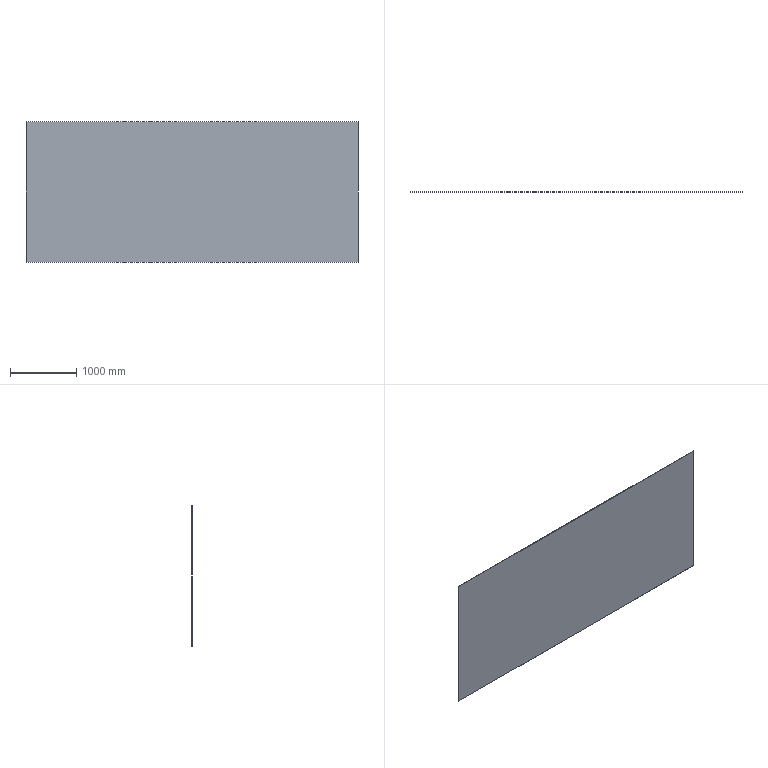Part | SolidWorks | features Extrusion 1 | 1 solid | 6 faces | box 5020 x 8 x 2120 mm | volume 85139200 mm3 | plane 6
STEP:
#1=CARTESIAN_POINT('',(2510.,0.,1060.));
#2=VERTEX_POINT('',#1);
#3=CARTESIAN_POINT('',(2510.,0.,-1060.));
#4=VERTEX_POINT('',#3);
#5=CARTESIAN_POINT('',(2510.,0.,1060.));
#6=DIRECTION('',(0.,0.,-1.));
#7=VECTOR('',#6,1000.);
#8=LINE('',#5,#7);
#9=EDGE_CURVE('',#2,#4,#8,.T.);
#10=ORIENTED_EDGE('',*,*,#9,.T.);
#11=CARTESIAN_POINT('',(2510.,8.,-1060.));
#12=VERTEX_POINT('',#11);
#13=CARTESIAN_POINT('',(2510.,8.,-1060.));
#14=DIRECTION('',(0.,-1.,0.));
#15=VECTOR('',#14,1000.);
#16=LINE('',#13,#15);
#17=EDGE_CURVE('',#12,#4,#16,.T.);
#18=ORIENTED_EDGE('',*,*,#17,.F.);
#19=CARTESIAN_POINT('',(2510.,8.,1060.));
#20=VERTEX_POINT('',#19);
#21=CARTESIAN_POINT('',(2510.,8.,1060.));
#22=DIRECTION('',(0.,0.,-1.));
#23=VECTOR('',#22,1000.);
#24=LINE('',#21,#23);
#25=EDGE_CURVE('',#20,#12,#24,.T.);
#26=ORIENTED_EDGE('',*,*,#25,.F.);
#27=CARTESIAN_POINT('',(2510.,8.,1060.));
#28=DIRECTION('',(0.,-1.,0.));
#29=VECTOR('',#28,1000.);
#30=LINE('',#27,#29);
#31=EDGE_CURVE('',#20,#2,#30,.T.);
#32=ORIENTED_EDGE('',*,*,#31,.T.);
#33=EDGE_LOOP('',(#10,#18,#26,#32));
#34=FACE_OUTER_BOUND('',#33,.T.);
#35=CARTESIAN_POINT('',(2510.,8.,1060.));
#36=DIRECTION('',(-1.,0.,0.));
#37=DIRECTION('',(0.,0.,1.));
#38=AXIS2_PLACEMENT_3D('',#35,#36,#37);
#39=PLANE('',#38);
#40=ADVANCED_FACE('',(#34),#39,.F.);
#41=CARTESIAN_POINT('',(-2510.,0.,-1060.));
#42=VERTEX_POINT('',#41);
#43=CARTESIAN_POINT('',(-2510.,0.,-1060.));
#44=DIRECTION('',(-1.,0.,0.));
#45=VECTOR('',#44,1000.);
#46=LINE('',#43,#45);
#47=EDGE_CURVE('',#4,#42,#46,.T.);
#48=ORIENTED_EDGE('',*,*,#47,.T.);
#49=CARTESIAN_POINT('',(-2510.,8.,-1060.));
#50=VERTEX_POINT('',#49);
#51=CARTESIAN_POINT('',(-2510.,8.,-1060.));
#52=DIRECTION('',(0.,-1.,0.));
#53=VECTOR('',#52,1000.);
#54=LINE('',#51,#53);
#55=EDGE_CURVE('',#50,#42,#54,.T.);
#56=ORIENTED_EDGE('',*,*,#55,.F.);
#57=CARTESIAN_POINT('',(-2510.,8.,-1060.));
#58=DIRECTION('',(-1.,0.,0.));
#59=VECTOR('',#58,1000.);
#60=LINE('',#57,#59);
#61=EDGE_CURVE('',#12,#50,#60,.T.);
#62=ORIENTED_EDGE('',*,*,#61,.F.);
#63=ORIENTED_EDGE('',*,*,#17,.T.);
#64=EDGE_LOOP('',(#48,#56,#62,#63));
#65=FACE_OUTER_BOUND('',#64,.T.);
#66=CARTESIAN_POINT('',(-2510.,8.,-1060.));
#67=DIRECTION('',(0.,0.,1.));
#68=DIRECTION('',(1.,0.,0.));
#69=AXIS2_PLACEMENT_3D('',#66,#67,#68);
#70=PLANE('',#69);
#71=ADVANCED_FACE('',(#65),#70,.F.);
#72=CARTESIAN_POINT('',(-2510.,0.,1060.));
#73=VERTEX_POINT('',#72);
#74=CARTESIAN_POINT('',(-2510.,0.,1060.));
#75=DIRECTION('',(0.,0.,1.));
#76=VECTOR('',#75,1000.);
#77=LINE('',#74,#76);
#78=EDGE_CURVE('',#42,#73,#77,.T.);
#79=ORIENTED_EDGE('',*,*,#78,.T.);
#80=CARTESIAN_POINT('',(-2510.,8.,1060.));
#81=VERTEX_POINT('',#80);
#82=CARTESIAN_POINT('',(-2510.,8.,1060.));
#83=DIRECTION('',(0.,-1.,0.));
#84=VECTOR('',#83,1000.);
#85=LINE('',#82,#84);
#86=EDGE_CURVE('',#81,#73,#85,.T.);
#87=ORIENTED_EDGE('',*,*,#86,.F.);
#88=CARTESIAN_POINT('',(-2510.,8.,1060.));
#89=DIRECTION('',(0.,0.,1.));
#90=VECTOR('',#89,1000.);
#91=LINE('',#88,#90);
#92=EDGE_CURVE('',#50,#81,#91,.T.);
#93=ORIENTED_EDGE('',*,*,#92,.F.);
#94=ORIENTED_EDGE('',*,*,#55,.T.);
#95=EDGE_LOOP('',(#79,#87,#93,#94));
#96=FACE_OUTER_BOUND('',#95,.T.);
#97=CARTESIAN_POINT('',(-2510.,8.,1060.));
#98=DIRECTION('',(1.,0.,0.));
#99=DIRECTION('',(0.,0.,-1.));
#100=AXIS2_PLACEMENT_3D('',#97,#98,#99);
#101=PLANE('',#100);
#102=ADVANCED_FACE('',(#96),#101,.F.);
#103=CARTESIAN_POINT('',(-2510.,0.,1060.));
#104=DIRECTION('',(1.,0.,0.));
#105=VECTOR('',#104,1000.);
#106=LINE('',#103,#105);
#107=EDGE_CURVE('',#73,#2,#106,.T.);
#108=ORIENTED_EDGE('',*,*,#107,.T.);
#109=ORIENTED_EDGE('',*,*,#31,.F.);
#110=CARTESIAN_POINT('',(-2510.,8.,1060.));
#111=DIRECTION('',(1.,0.,0.));
#112=VECTOR('',#111,1000.);
#113=LINE('',#110,#112);
#114=EDGE_CURVE('',#81,#20,#113,.T.);
#115=ORIENTED_EDGE('',*,*,#114,.F.);
#116=ORIENTED_EDGE('',*,*,#86,.T.);
#117=EDGE_LOOP('',(#108,#109,#115,#116));
#118=FACE_OUTER_BOUND('',#117,.T.);
#119=CARTESIAN_POINT('',(-2510.,8.,1060.));
#120=DIRECTION('',(0.,0.,-1.));
#121=DIRECTION('',(-1.,0.,0.));
#122=AXIS2_PLACEMENT_3D('',#119,#120,#121);
#123=PLANE('',#122);
#124=ADVANCED_FACE('',(#118),#123,.F.);
#125=ORIENTED_EDGE('',*,*,#25,.T.);
#126=ORIENTED_EDGE('',*,*,#61,.T.);
#127=ORIENTED_EDGE('',*,*,#92,.T.);
#128=ORIENTED_EDGE('',*,*,#114,.T.);
#129=EDGE_LOOP('',(#125,#126,#127,#128));
#130=FACE_OUTER_BOUND('',#129,.T.);
#131=CARTESIAN_POINT('',(0.,8.,0.));
#132=DIRECTION('',(0.,-1.,0.));
#133=DIRECTION('',(0.,0.,-1.));
#134=AXIS2_PLACEMENT_3D('',#131,#132,#133);
#135=PLANE('',#134);
#136=ADVANCED_FACE('',(#130),#135,.F.);
#137=ORIENTED_EDGE('',*,*,#9,.F.);
#138=ORIENTED_EDGE('',*,*,#107,.F.);
#139=ORIENTED_EDGE('',*,*,#78,.F.);
#140=ORIENTED_EDGE('',*,*,#47,.F.);
#141=EDGE_LOOP('',(#137,#138,#139,#140));
#142=FACE_OUTER_BOUND('',#141,.T.);
#143=CARTESIAN_POINT('',(0.,0.,0.));
#144=DIRECTION('',(0.,-1.,0.));
#145=DIRECTION('',(0.,0.,-1.));
#146=AXIS2_PLACEMENT_3D('',#143,#144,#145);
#147=PLANE('',#146);
#148=ADVANCED_FACE('',(#142),#147,.T.);
#149=CLOSED_SHELL('',(#40,#71,#102,#124,#136,#148));
#150=MANIFOLD_SOLID_BREP('',#149);
#151=CARTESIAN_POINT('',(0.,0.,0.));
#152=DIRECTION('',(0.,0.,1.));
#153=DIRECTION('',(1.,0.,0.));
#154=AXIS2_PLACEMENT_3D('',#151,#152,#153);
#155=(LENGTH_UNIT()NAMED_UNIT(*)SI_UNIT(.MILLI.,.METRE.));
#156=UNCERTAINTY_MEASURE_WITH_UNIT(LENGTH_MEASURE(0.00001),#155,'','');
#157=(NAMED_UNIT(*)PLANE_ANGLE_UNIT()SI_UNIT($,.RADIAN.));
#158=(NAMED_UNIT(*)SI_UNIT($,.STERADIAN.)SOLID_ANGLE_UNIT());
#159=(GEOMETRIC_REPRESENTATION_CONTEXT(3)GLOBAL_UNCERTAINTY_ASSIGNED_CONTEXT((#156))GLOBAL_UNIT_ASSIGNED_CONTEXT((#155,#157,#158))REPRESENTATION_CONTEXT('',''));
#160=ADVANCED_BREP_SHAPE_REPRESENTATION('',(#150,#154),#159);